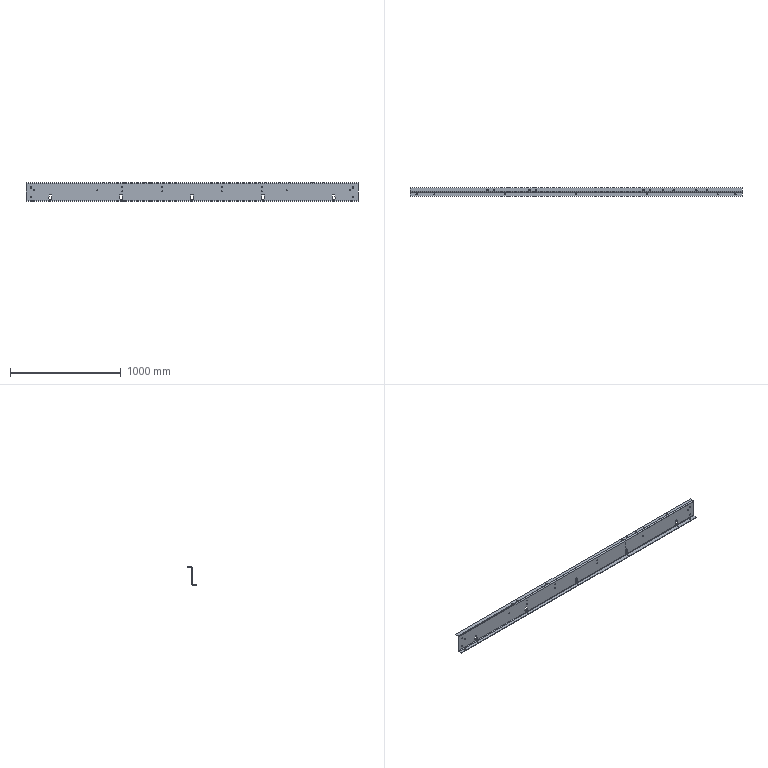Part | SolidWorks | features BaseBody 1 | 1 solid | 115 faces | box 3000 x 75 x 170 mm | volume 3462019 mm3 | cylinder 95 | plane 20 | commonest cylinder face diameters 12 x28 10 x20 9 x16 7 x10 30 x10 25 x5